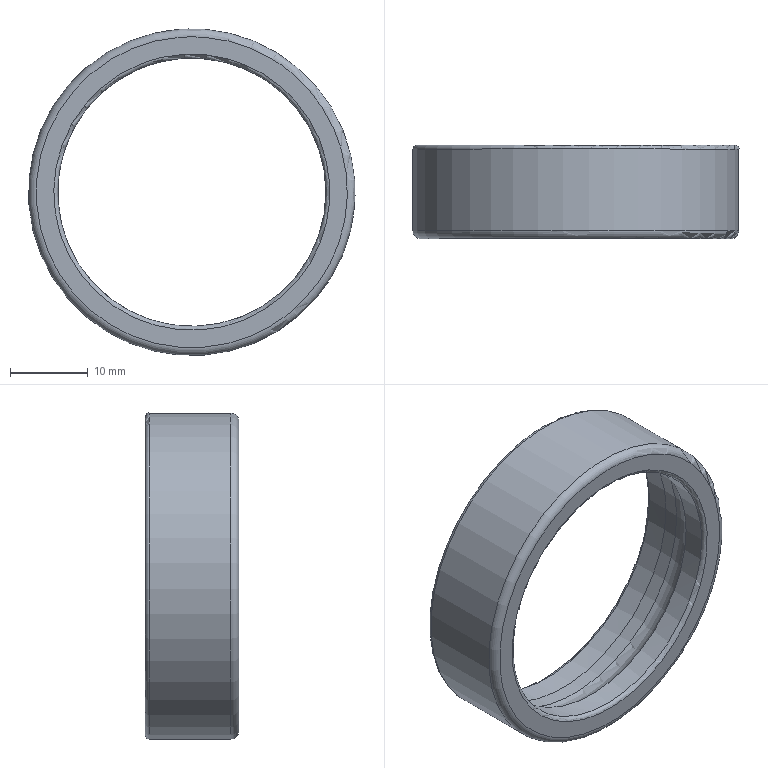Part | STEP file | BK-20_id1314_x_t | 1 solid | 11 faces | box 42 x 12 x 42 mm | volume 3939 mm3 | torus 5 | cylinder 3 | plane 2 | cone 1 | commonest cylinder face diameters 34.5 x1 37.5 x1 42 x1